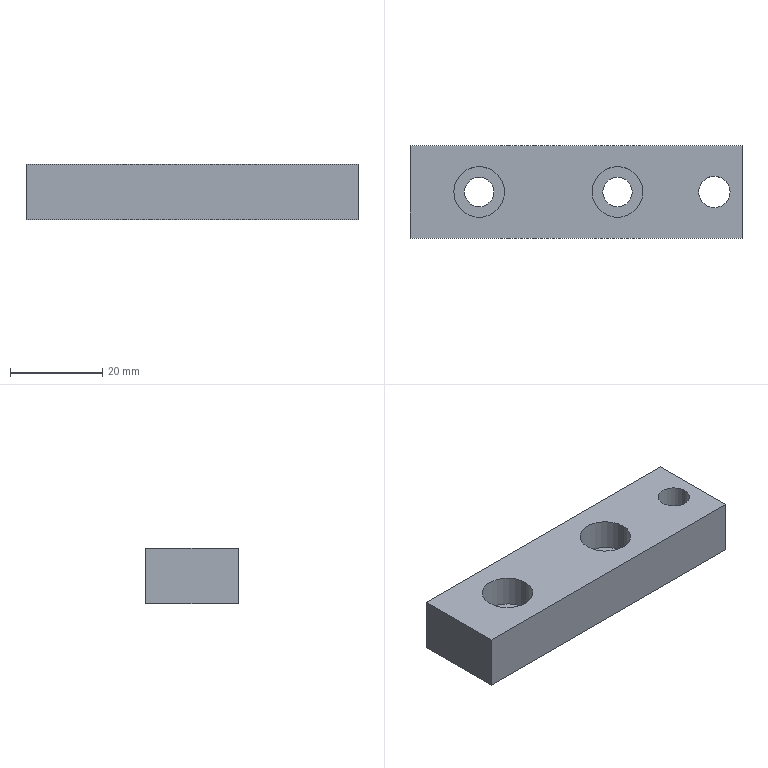Part | STEP file | Tensioning block | 1 solid | 18 faces | box 72 x 20 x 12 mm | volume 15217 mm3 | cylinder 10 | plane 8 | commonest cylinder face diameters 6.4 x4 11 x4 6.8 x2
STEP:
#1=CARTESIAN_POINT('',(0.,0.,0.));
#2=DIRECTION('',(0.,0.,1.));
#3=DIRECTION('',(1.,0.,0.));
#4=AXIS2_PLACEMENT_3D('',#1,#2,#3);
#5=CARTESIAN_POINT('',(33.4,0.,0.));
#6=VERTEX_POINT('',#5);
#7=CARTESIAN_POINT('',(33.4,0.,12.));
#8=VERTEX_POINT('',#7);
#9=CARTESIAN_POINT('',(33.4,0.,12.));
#10=DIRECTION('',(0.,0.,1.));
#11=VECTOR('',#10,1.);
#12=LINE('',#9,#11);
#13=CARTESIAN_POINT('',(30.,0.,12.));
#14=DIRECTION('',(0.,0.,1.));
#15=DIRECTION('',(1.,0.,0.));
#16=AXIS2_PLACEMENT_3D('',#13,#14,#15);
#17=CYLINDRICAL_SURFACE('',#16,3.4);
#18=CARTESIAN_POINT('',(6.283,0.));
#19=DIRECTION('',(0.,1.));
#20=VECTOR('',#19,1.);
#21=LINE('',#18,#20);
#22=(GEOMETRIC_REPRESENTATION_CONTEXT(2)PARAMETRIC_REPRESENTATION_CONTEXT()REPRESENTATION_CONTEXT('',''));
#23=DEFINITIONAL_REPRESENTATION('',(#21),#22);
#24=PCURVE('',#17,#23);
#25=CARTESIAN_POINT('',(30.,0.,12.));
#26=DIRECTION('',(0.,0.,1.));
#27=DIRECTION('',(1.,0.,0.));
#28=AXIS2_PLACEMENT_3D('',#25,#26,#27);
#29=CYLINDRICAL_SURFACE('',#28,3.4);
#30=CARTESIAN_POINT('',(0.,0.));
#31=DIRECTION('',(0.,1.));
#32=VECTOR('',#31,1.);
#33=LINE('',#30,#32);
#34=(GEOMETRIC_REPRESENTATION_CONTEXT(2)PARAMETRIC_REPRESENTATION_CONTEXT()REPRESENTATION_CONTEXT('',''));
#35=DEFINITIONAL_REPRESENTATION('',(#33),#34);
#36=PCURVE('',#29,#35);
#37=SURFACE_CURVE('',#12,(#24,#36),.PCURVE_S1.);
#38=EDGE_CURVE('',#6,#8,#37,.T.);
#39=ORIENTED_EDGE('',*,*,#38,.T.);
#40=CARTESIAN_POINT('',(26.6,0.,12.));
#41=VERTEX_POINT('',#40);
#42=CARTESIAN_POINT('',(30.,0.,12.));
#43=DIRECTION('',(0.,0.,1.));
#44=DIRECTION('',(1.,0.,0.));
#45=AXIS2_PLACEMENT_3D('',#42,#43,#44);
#46=CIRCLE('',#45,3.4);
#47=CARTESIAN_POINT('',(0.,0.));
#48=DIRECTION('',(1.,0.));
#49=VECTOR('',#48,1.);
#50=LINE('',#47,#49);
#51=(GEOMETRIC_REPRESENTATION_CONTEXT(2)PARAMETRIC_REPRESENTATION_CONTEXT()REPRESENTATION_CONTEXT('',''));
#52=DEFINITIONAL_REPRESENTATION('',(#50),#51);
#53=PCURVE('',#17,#52);
#54=CARTESIAN_POINT('',(0.,0.,12.));
#55=DIRECTION('',(0.,0.,1.));
#56=DIRECTION('',(1.,0.,0.));
#57=AXIS2_PLACEMENT_3D('',#54,#55,#56);
#58=PLANE('',#57);
#59=CARTESIAN_POINT('',(30.,0.));
#60=DIRECTION('',(1.,0.));
#61=AXIS2_PLACEMENT_2D('',#59,#60);
#62=CIRCLE('',#61,3.4);
#63=(GEOMETRIC_REPRESENTATION_CONTEXT(2)PARAMETRIC_REPRESENTATION_CONTEXT()REPRESENTATION_CONTEXT('',''));
#64=DEFINITIONAL_REPRESENTATION('',(#62),#63);
#65=PCURVE('',#58,#64);
#66=SURFACE_CURVE('',#46,(#53,#65),.PCURVE_S1.);
#67=EDGE_CURVE('',#41,#8,#66,.T.);
#68=ORIENTED_EDGE('',*,*,#67,.F.);
#69=CARTESIAN_POINT('',(26.6,0.,0.));
#70=VERTEX_POINT('',#69);
#71=CARTESIAN_POINT('',(26.6,0.,12.));
#72=DIRECTION('',(0.,0.,1.));
#73=VECTOR('',#72,1.);
#74=LINE('',#71,#73);
#75=CARTESIAN_POINT('',(3.142,0.));
#76=DIRECTION('',(0.,1.));
#77=VECTOR('',#76,1.);
#78=LINE('',#75,#77);
#79=(GEOMETRIC_REPRESENTATION_CONTEXT(2)PARAMETRIC_REPRESENTATION_CONTEXT()REPRESENTATION_CONTEXT('',''));
#80=DEFINITIONAL_REPRESENTATION('',(#78),#79);
#81=PCURVE('',#17,#80);
#82=CARTESIAN_POINT('',(3.142,0.));
#83=DIRECTION('',(0.,1.));
#84=VECTOR('',#83,1.);
#85=LINE('',#82,#84);
#86=(GEOMETRIC_REPRESENTATION_CONTEXT(2)PARAMETRIC_REPRESENTATION_CONTEXT()REPRESENTATION_CONTEXT('',''));
#87=DEFINITIONAL_REPRESENTATION('',(#85),#86);
#88=PCURVE('',#29,#87);
#89=SURFACE_CURVE('',#74,(#81,#88),.PCURVE_S1.);
#90=EDGE_CURVE('',#70,#41,#89,.T.);
#91=ORIENTED_EDGE('',*,*,#90,.F.);
#92=CARTESIAN_POINT('',(30.,0.,0.));
#93=DIRECTION('',(0.,0.,1.));
#94=DIRECTION('',(1.,0.,0.));
#95=AXIS2_PLACEMENT_3D('',#92,#93,#94);
#96=CIRCLE('',#95,3.4);
#97=CARTESIAN_POINT('',(0.,-12.));
#98=DIRECTION('',(1.,0.));
#99=VECTOR('',#98,1.);
#100=LINE('',#97,#99);
#101=(GEOMETRIC_REPRESENTATION_CONTEXT(2)PARAMETRIC_REPRESENTATION_CONTEXT()REPRESENTATION_CONTEXT('',''));
#102=DEFINITIONAL_REPRESENTATION('',(#100),#101);
#103=PCURVE('',#17,#102);
#104=CARTESIAN_POINT('',(0.,0.,0.));
#105=DIRECTION('',(0.,0.,1.));
#106=DIRECTION('',(1.,0.,0.));
#107=AXIS2_PLACEMENT_3D('',#104,#105,#106);
#108=PLANE('',#107);
#109=CARTESIAN_POINT('',(30.,0.));
#110=DIRECTION('',(1.,0.));
#111=AXIS2_PLACEMENT_2D('',#109,#110);
#112=CIRCLE('',#111,3.4);
#113=(GEOMETRIC_REPRESENTATION_CONTEXT(2)PARAMETRIC_REPRESENTATION_CONTEXT()REPRESENTATION_CONTEXT('',''));
#114=DEFINITIONAL_REPRESENTATION('',(#112),#113);
#115=PCURVE('',#108,#114);
#116=SURFACE_CURVE('',#96,(#103,#115),.PCURVE_S1.);
#117=EDGE_CURVE('',#70,#6,#116,.T.);
#118=ORIENTED_EDGE('',*,*,#117,.T.);
#119=EDGE_LOOP('',(#39,#68,#91,#118));
#120=FACE_BOUND('',#119,.F.);
#121=ADVANCED_FACE('',(#120),#17,.F.);
#122=CARTESIAN_POINT('',(-15.5,0.,5.2));
#123=VERTEX_POINT('',#122);
#124=CARTESIAN_POINT('',(-15.5,0.,12.));
#125=VERTEX_POINT('',#124);
#126=CARTESIAN_POINT('',(-15.5,0.,12.));
#127=DIRECTION('',(0.,0.,1.));
#128=VECTOR('',#127,1.);
#129=LINE('',#126,#128);
#130=CARTESIAN_POINT('',(-21.,0.,12.));
#131=DIRECTION('',(0.,0.,1.));
#132=DIRECTION('',(1.,0.,0.));
#133=AXIS2_PLACEMENT_3D('',#130,#131,#132);
#134=CYLINDRICAL_SURFACE('',#133,5.5);
#135=CARTESIAN_POINT('',(6.283,0.));
#136=DIRECTION('',(0.,1.));
#137=VECTOR('',#136,1.);
#138=LINE('',#135,#137);
#139=(GEOMETRIC_REPRESENTATION_CONTEXT(2)PARAMETRIC_REPRESENTATION_CONTEXT()REPRESENTATION_CONTEXT('',''));
#140=DEFINITIONAL_REPRESENTATION('',(#138),#139);
#141=PCURVE('',#134,#140);
#142=CARTESIAN_POINT('',(-21.,0.,12.));
#143=DIRECTION('',(0.,0.,1.));
#144=DIRECTION('',(1.,0.,0.));
#145=AXIS2_PLACEMENT_3D('',#142,#143,#144);
#146=CYLINDRICAL_SURFACE('',#145,5.5);
#147=CARTESIAN_POINT('',(0.,0.));
#148=DIRECTION('',(0.,1.));
#149=VECTOR('',#148,1.);
#150=LINE('',#147,#149);
#151=(GEOMETRIC_REPRESENTATION_CONTEXT(2)PARAMETRIC_REPRESENTATION_CONTEXT()REPRESENTATION_CONTEXT('',''));
#152=DEFINITIONAL_REPRESENTATION('',(#150),#151);
#153=PCURVE('',#146,#152);
#154=SURFACE_CURVE('',#129,(#141,#153),.PCURVE_S1.);
#155=EDGE_CURVE('',#123,#125,#154,.T.);
#156=ORIENTED_EDGE('',*,*,#155,.T.);
#157=CARTESIAN_POINT('',(-26.5,0.,12.));
#158=VERTEX_POINT('',#157);
#159=CARTESIAN_POINT('',(-21.,0.,12.));
#160=DIRECTION('',(0.,0.,1.));
#161=DIRECTION('',(1.,0.,0.));
#162=AXIS2_PLACEMENT_3D('',#159,#160,#161);
#163=CIRCLE('',#162,5.5);
#164=CARTESIAN_POINT('',(0.,0.));
#165=DIRECTION('',(1.,0.));
#166=VECTOR('',#165,1.);
#167=LINE('',#164,#166);
#168=(GEOMETRIC_REPRESENTATION_CONTEXT(2)PARAMETRIC_REPRESENTATION_CONTEXT()REPRESENTATION_CONTEXT('',''));
#169=DEFINITIONAL_REPRESENTATION('',(#167),#168);
#170=PCURVE('',#134,#169);
#171=CARTESIAN_POINT('',(-21.,0.));
#172=DIRECTION('',(1.,0.));
#173=AXIS2_PLACEMENT_2D('',#171,#172);
#174=CIRCLE('',#173,5.5);
#175=(GEOMETRIC_REPRESENTATION_CONTEXT(2)PARAMETRIC_REPRESENTATION_CONTEXT()REPRESENTATION_CONTEXT('',''));
#176=DEFINITIONAL_REPRESENTATION('',(#174),#175);
#177=PCURVE('',#58,#176);
#178=SURFACE_CURVE('',#163,(#170,#177),.PCURVE_S1.);
#179=EDGE_CURVE('',#158,#125,#178,.T.);
#180=ORIENTED_EDGE('',*,*,#179,.F.);
#181=CARTESIAN_POINT('',(-26.5,0.,5.2));
#182=VERTEX_POINT('',#181);
#183=CARTESIAN_POINT('',(-26.5,0.,12.));
#184=DIRECTION('',(0.,0.,1.));
#185=VECTOR('',#184,1.);
#186=LINE('',#183,#185);
#187=CARTESIAN_POINT('',(3.142,0.));
#188=DIRECTION('',(0.,1.));
#189=VECTOR('',#188,1.);
#190=LINE('',#187,#189);
#191=(GEOMETRIC_REPRESENTATION_CONTEXT(2)PARAMETRIC_REPRESENTATION_CONTEXT()REPRESENTATION_CONTEXT('',''));
#192=DEFINITIONAL_REPRESENTATION('',(#190),#191);
#193=PCURVE('',#134,#192);
#194=CARTESIAN_POINT('',(3.142,0.));
#195=DIRECTION('',(0.,1.));
#196=VECTOR('',#195,1.);
#197=LINE('',#194,#196);
#198=(GEOMETRIC_REPRESENTATION_CONTEXT(2)PARAMETRIC_REPRESENTATION_CONTEXT()REPRESENTATION_CONTEXT('',''));
#199=DEFINITIONAL_REPRESENTATION('',(#197),#198);
#200=PCURVE('',#146,#199);
#201=SURFACE_CURVE('',#186,(#193,#200),.PCURVE_S1.);
#202=EDGE_CURVE('',#182,#158,#201,.T.);
#203=ORIENTED_EDGE('',*,*,#202,.F.);
#204=CARTESIAN_POINT('',(-21.,0.,5.2));
#205=DIRECTION('',(0.,0.,1.));
#206=DIRECTION('',(1.,0.,0.));
#207=AXIS2_PLACEMENT_3D('',#204,#205,#206);
#208=CIRCLE('',#207,5.5);
#209=CARTESIAN_POINT('',(0.,-6.8));
#210=DIRECTION('',(1.,0.));
#211=VECTOR('',#210,1.);
#212=LINE('',#209,#211);
#213=(GEOMETRIC_REPRESENTATION_CONTEXT(2)PARAMETRIC_REPRESENTATION_CONTEXT()REPRESENTATION_CONTEXT('',''));
#214=DEFINITIONAL_REPRESENTATION('',(#212),#213);
#215=PCURVE('',#134,#214);
#216=CARTESIAN_POINT('',(-17.8,0.,5.2));
#217=DIRECTION('',(0.,0.,-1.));
#218=DIRECTION('',(-1.,0.,0.));
#219=AXIS2_PLACEMENT_3D('',#216,#217,#218);
#220=PLANE('',#219);
#221=CARTESIAN_POINT('',(-2.3,0.));
#222=CARTESIAN_POINT('',(-2.3,9.526));
#223=CARTESIAN_POINT('',(5.95,4.763));
#224=CARTESIAN_POINT('',(14.2,0.));
#225=CARTESIAN_POINT('',(5.95,-4.763));
#226=CARTESIAN_POINT('',(-2.3,-9.526));
#227=CARTESIAN_POINT('',(-2.3,0.));
#228=(BOUNDED_CURVE()B_SPLINE_CURVE(2,(#221,#222,#223,#224,#225,#226,#227),.UNSPECIFIED.,.T.,.F.)B_SPLINE_CURVE_WITH_KNOTS((1,2,2,2,2,1),(-2.094,0.,2.094,4.189,6.283,8.378),.UNSPECIFIED.)CURVE()GEOMETRIC_REPRESENTATION_ITEM()RATIONAL_B_SPLINE_CURVE((1.,0.5,1.,0.5,1.,0.5,1.))REPRESENTATION_ITEM(''));
#229=(GEOMETRIC_REPRESENTATION_CONTEXT(2)PARAMETRIC_REPRESENTATION_CONTEXT()REPRESENTATION_CONTEXT('',''));
#230=DEFINITIONAL_REPRESENTATION('',(#228),#229);
#231=PCURVE('',#220,#230);
#232=SURFACE_CURVE('',#208,(#215,#231),.PCURVE_S1.);
#233=EDGE_CURVE('',#182,#123,#232,.T.);
#234=ORIENTED_EDGE('',*,*,#233,.T.);
#235=EDGE_LOOP('',(#156,#180,#203,#234));
#236=FACE_BOUND('',#235,.F.);
#237=ADVANCED_FACE('',(#236),#134,.F.);
#238=CARTESIAN_POINT('',(-17.8,0.,0.));
#239=VERTEX_POINT('',#238);
#240=CARTESIAN_POINT('',(-17.8,0.,5.2));
#241=VERTEX_POINT('',#240);
#242=CARTESIAN_POINT('',(-17.8,0.,12.));
#243=DIRECTION('',(0.,0.,1.));
#244=VECTOR('',#243,1.);
#245=LINE('',#242,#244);
#246=CARTESIAN_POINT('',(-21.,0.,12.));
#247=DIRECTION('',(0.,0.,1.));
#248=DIRECTION('',(1.,0.,0.));
#249=AXIS2_PLACEMENT_3D('',#246,#247,#248);
#250=CYLINDRICAL_SURFACE('',#249,3.2);
#251=CARTESIAN_POINT('',(6.283,0.));
#252=DIRECTION('',(0.,1.));
#253=VECTOR('',#252,1.);
#254=LINE('',#251,#253);
#255=(GEOMETRIC_REPRESENTATION_CONTEXT(2)PARAMETRIC_REPRESENTATION_CONTEXT()REPRESENTATION_CONTEXT('',''));
#256=DEFINITIONAL_REPRESENTATION('',(#254),#255);
#257=PCURVE('',#250,#256);
#258=CARTESIAN_POINT('',(-21.,0.,12.));
#259=DIRECTION('',(0.,0.,1.));
#260=DIRECTION('',(1.,0.,0.));
#261=AXIS2_PLACEMENT_3D('',#258,#259,#260);
#262=CYLINDRICAL_SURFACE('',#261,3.2);
#263=CARTESIAN_POINT('',(0.,0.));
#264=DIRECTION('',(0.,1.));
#265=VECTOR('',#264,1.);
#266=LINE('',#263,#265);
#267=(GEOMETRIC_REPRESENTATION_CONTEXT(2)PARAMETRIC_REPRESENTATION_CONTEXT()REPRESENTATION_CONTEXT('',''));
#268=DEFINITIONAL_REPRESENTATION('',(#266),#267);
#269=PCURVE('',#262,#268);
#270=SURFACE_CURVE('',#245,(#257,#269),.PCURVE_S1.);
#271=EDGE_CURVE('',#239,#241,#270,.T.);
#272=ORIENTED_EDGE('',*,*,#271,.T.);
#273=CARTESIAN_POINT('',(-24.2,0.,5.2));
#274=VERTEX_POINT('',#273);
#275=CARTESIAN_POINT('',(-21.,0.,5.2));
#276=DIRECTION('',(0.,0.,1.));
#277=DIRECTION('',(1.,0.,0.));
#278=AXIS2_PLACEMENT_3D('',#275,#276,#277);
#279=CIRCLE('',#278,3.2);
#280=CARTESIAN_POINT('',(0.,-6.8));
#281=DIRECTION('',(1.,0.));
#282=VECTOR('',#281,1.);
#283=LINE('',#280,#282);
#284=(GEOMETRIC_REPRESENTATION_CONTEXT(2)PARAMETRIC_REPRESENTATION_CONTEXT()REPRESENTATION_CONTEXT('',''));
#285=DEFINITIONAL_REPRESENTATION('',(#283),#284);
#286=PCURVE('',#250,#285);
#287=CARTESIAN_POINT('',(0.,0.));
#288=CARTESIAN_POINT('',(0.,5.543));
#289=CARTESIAN_POINT('',(4.8,2.771));
#290=CARTESIAN_POINT('',(9.6,0.));
#291=CARTESIAN_POINT('',(4.8,-2.771));
#292=CARTESIAN_POINT('',(0.,-5.543));
#293=CARTESIAN_POINT('',(0.,0.));
#294=(BOUNDED_CURVE()B_SPLINE_CURVE(2,(#287,#288,#289,#290,#291,#292,#293),.UNSPECIFIED.,.T.,.F.)B_SPLINE_CURVE_WITH_KNOTS((1,2,2,2,2,1),(-2.094,0.,2.094,4.189,6.283,8.378),.UNSPECIFIED.)CURVE()GEOMETRIC_REPRESENTATION_ITEM()RATIONAL_B_SPLINE_CURVE((1.,0.5,1.,0.5,1.,0.5,1.))REPRESENTATION_ITEM(''));
#295=(GEOMETRIC_REPRESENTATION_CONTEXT(2)PARAMETRIC_REPRESENTATION_CONTEXT()REPRESENTATION_CONTEXT('',''));
#296=DEFINITIONAL_REPRESENTATION('',(#294),#295);
#297=PCURVE('',#220,#296);
#298=SURFACE_CURVE('',#279,(#286,#297),.PCURVE_S1.);
#299=EDGE_CURVE('',#274,#241,#298,.T.);
#300=ORIENTED_EDGE('',*,*,#299,.F.);
#301=CARTESIAN_POINT('',(-24.2,0.,0.));
#302=VERTEX_POINT('',#301);
#303=CARTESIAN_POINT('',(-24.2,0.,12.));
#304=DIRECTION('',(0.,0.,1.));
#305=VECTOR('',#304,1.);
#306=LINE('',#303,#305);
#307=CARTESIAN_POINT('',(3.142,0.));
#308=DIRECTION('',(0.,1.));
#309=VECTOR('',#308,1.);
#310=LINE('',#307,#309);
#311=(GEOMETRIC_REPRESENTATION_CONTEXT(2)PARAMETRIC_REPRESENTATION_CONTEXT()REPRESENTATION_CONTEXT('',''));
#312=DEFINITIONAL_REPRESENTATION('',(#310),#311);
#313=PCURVE('',#250,#312);
#314=CARTESIAN_POINT('',(3.142,0.));
#315=DIRECTION('',(0.,1.));
#316=VECTOR('',#315,1.);
#317=LINE('',#314,#316);
#318=(GEOMETRIC_REPRESENTATION_CONTEXT(2)PARAMETRIC_REPRESENTATION_CONTEXT()REPRESENTATION_CONTEXT('',''));
#319=DEFINITIONAL_REPRESENTATION('',(#317),#318);
#320=PCURVE('',#262,#319);
#321=SURFACE_CURVE('',#306,(#313,#320),.PCURVE_S1.);
#322=EDGE_CURVE('',#302,#274,#321,.T.);
#323=ORIENTED_EDGE('',*,*,#322,.F.);
#324=CARTESIAN_POINT('',(-21.,0.,0.));
#325=DIRECTION('',(0.,0.,1.));
#326=DIRECTION('',(1.,0.,0.));
#327=AXIS2_PLACEMENT_3D('',#324,#325,#326);
#328=CIRCLE('',#327,3.2);
#329=CARTESIAN_POINT('',(0.,-12.));
#330=DIRECTION('',(1.,0.));
#331=VECTOR('',#330,1.);
#332=LINE('',#329,#331);
#333=(GEOMETRIC_REPRESENTATION_CONTEXT(2)PARAMETRIC_REPRESENTATION_CONTEXT()REPRESENTATION_CONTEXT('',''));
#334=DEFINITIONAL_REPRESENTATION('',(#332),#333);
#335=PCURVE('',#250,#334);
#336=CARTESIAN_POINT('',(-21.,0.));
#337=DIRECTION('',(1.,0.));
#338=AXIS2_PLACEMENT_2D('',#336,#337);
#339=CIRCLE('',#338,3.2);
#340=(GEOMETRIC_REPRESENTATION_CONTEXT(2)PARAMETRIC_REPRESENTATION_CONTEXT()REPRESENTATION_CONTEXT('',''));
#341=DEFINITIONAL_REPRESENTATION('',(#339),#340);
#342=PCURVE('',#108,#341);
#343=SURFACE_CURVE('',#328,(#335,#342),.PCURVE_S1.);
#344=EDGE_CURVE('',#302,#239,#343,.T.);
#345=ORIENTED_EDGE('',*,*,#344,.T.);
#346=EDGE_LOOP('',(#272,#300,#323,#345));
#347=FACE_BOUND('',#346,.F.);
#348=ADVANCED_FACE('',(#347),#250,.F.);
#349=CARTESIAN_POINT('',(14.5,0.,5.2));
#350=VERTEX_POINT('',#349);
#351=CARTESIAN_POINT('',(14.5,0.,12.));
#352=VERTEX_POINT('',#351);
#353=CARTESIAN_POINT('',(14.5,0.,12.));
#354=DIRECTION('',(0.,0.,1.));
#355=VECTOR('',#354,1.);
#356=LINE('',#353,#355);
#357=CARTESIAN_POINT('',(9.,0.,12.));
#358=DIRECTION('',(0.,0.,1.));
#359=DIRECTION('',(1.,0.,0.));
#360=AXIS2_PLACEMENT_3D('',#357,#358,#359);
#361=CYLINDRICAL_SURFACE('',#360,5.5);
#362=CARTESIAN_POINT('',(6.283,0.));
#363=DIRECTION('',(0.,1.));
#364=VECTOR('',#363,1.);
#365=LINE('',#362,#364);
#366=(GEOMETRIC_REPRESENTATION_CONTEXT(2)PARAMETRIC_REPRESENTATION_CONTEXT()REPRESENTATION_CONTEXT('',''));
#367=DEFINITIONAL_REPRESENTATION('',(#365),#366);
#368=PCURVE('',#361,#367);
#369=CARTESIAN_POINT('',(9.,0.,12.));
#370=DIRECTION('',(0.,0.,1.));
#371=DIRECTION('',(1.,0.,0.));
#372=AXIS2_PLACEMENT_3D('',#369,#370,#371);
#373=CYLINDRICAL_SURFACE('',#372,5.5);
#374=CARTESIAN_POINT('',(0.,0.));
#375=DIRECTION('',(0.,1.));
#376=VECTOR('',#375,1.);
#377=LINE('',#374,#376);
#378=(GEOMETRIC_REPRESENTATION_CONTEXT(2)PARAMETRIC_REPRESENTATION_CONTEXT()REPRESENTATION_CONTEXT('',''));
#379=DEFINITIONAL_REPRESENTATION('',(#377),#378);
#380=PCURVE('',#373,#379);
#381=SURFACE_CURVE('',#356,(#368,#380),.PCURVE_S1.);
#382=EDGE_CURVE('',#350,#352,#381,.T.);
#383=ORIENTED_EDGE('',*,*,#382,.T.);
#384=CARTESIAN_POINT('',(3.5,0.,12.));
#385=VERTEX_POINT('',#384);
#386=CARTESIAN_POINT('',(9.,0.,12.));
#387=DIRECTION('',(0.,0.,1.));
#388=DIRECTION('',(1.,0.,0.));
#389=AXIS2_PLACEMENT_3D('',#386,#387,#388);
#390=CIRCLE('',#389,5.5);
#391=CARTESIAN_POINT('',(0.,0.));
#392=DIRECTION('',(1.,0.));
#393=VECTOR('',#392,1.);
#394=LINE('',#391,#393);
#395=(GEOMETRIC_REPRESENTATION_CONTEXT(2)PARAMETRIC_REPRESENTATION_CONTEXT()REPRESENTATION_CONTEXT('',''));
#396=DEFINITIONAL_REPRESENTATION('',(#394),#395);
#397=PCURVE('',#361,#396);
#398=CARTESIAN_POINT('',(9.,0.));
#399=DIRECTION('',(1.,0.));
#400=AXIS2_PLACEMENT_2D('',#398,#399);
#401=CIRCLE('',#400,5.5);
#402=(GEOMETRIC_REPRESENTATION_CONTEXT(2)PARAMETRIC_REPRESENTATION_CONTEXT()REPRESENTATION_CONTEXT('',''));
#403=DEFINITIONAL_REPRESENTATION('',(#401),#402);
#404=PCURVE('',#58,#403);
#405=SURFACE_CURVE('',#390,(#397,#404),.PCURVE_S1.);
#406=EDGE_CURVE('',#385,#352,#405,.T.);
#407=ORIENTED_EDGE('',*,*,#406,.F.);
#408=CARTESIAN_POINT('',(3.5,0.,5.2));
#409=VERTEX_POINT('',#408);
#410=CARTESIAN_POINT('',(3.5,0.,12.));
#411=DIRECTION('',(0.,0.,1.));
#412=VECTOR('',#411,1.);
#413=LINE('',#410,#412);
#414=CARTESIAN_POINT('',(3.142,0.));
#415=DIRECTION('',(0.,1.));
#416=VECTOR('',#415,1.);
#417=LINE('',#414,#416);
#418=(GEOMETRIC_REPRESENTATION_CONTEXT(2)PARAMETRIC_REPRESENTATION_CONTEXT()REPRESENTATION_CONTEXT('',''));
#419=DEFINITIONAL_REPRESENTATION('',(#417),#418);
#420=PCURVE('',#361,#419);
#421=CARTESIAN_POINT('',(3.142,0.));
#422=DIRECTION('',(0.,1.));
#423=VECTOR('',#422,1.);
#424=LINE('',#421,#423);
#425=(GEOMETRIC_REPRESENTATION_CONTEXT(2)PARAMETRIC_REPRESENTATION_CONTEXT()REPRESENTATION_CONTEXT('',''));
#426=DEFINITIONAL_REPRESENTATION('',(#424),#425);
#427=PCURVE('',#373,#426);
#428=SURFACE_CURVE('',#413,(#420,#427),.PCURVE_S1.);
#429=EDGE_CURVE('',#409,#385,#428,.T.);
#430=ORIENTED_EDGE('',*,*,#429,.F.);
#431=CARTESIAN_POINT('',(9.,0.,5.2));
#432=DIRECTION('',(0.,0.,1.));
#433=DIRECTION('',(1.,0.,0.));
#434=AXIS2_PLACEMENT_3D('',#431,#432,#433);
#435=CIRCLE('',#434,5.5);
#436=CARTESIAN_POINT('',(0.,-6.8));
#437=DIRECTION('',(1.,0.));
#438=VECTOR('',#437,1.);
#439=LINE('',#436,#438);
#440=(GEOMETRIC_REPRESENTATION_CONTEXT(2)PARAMETRIC_REPRESENTATION_CONTEXT()REPRESENTATION_CONTEXT('',''));
#441=DEFINITIONAL_REPRESENTATION('',(#439),#440);
#442=PCURVE('',#361,#441);
#443=CARTESIAN_POINT('',(12.2,0.,5.2));
#444=DIRECTION('',(0.,0.,-1.));
#445=DIRECTION('',(-1.,0.,0.));
#446=AXIS2_PLACEMENT_3D('',#443,#444,#445);
#447=PLANE('',#446);
#448=CARTESIAN_POINT('',(-2.3,0.));
#449=CARTESIAN_POINT('',(-2.3,9.526));
#450=CARTESIAN_POINT('',(5.95,4.763));
#451=CARTESIAN_POINT('',(14.2,0.));
#452=CARTESIAN_POINT('',(5.95,-4.763));
#453=CARTESIAN_POINT('',(-2.3,-9.526));
#454=CARTESIAN_POINT('',(-2.3,0.));
#455=(BOUNDED_CURVE()B_SPLINE_CURVE(2,(#448,#449,#450,#451,#452,#453,#454),.UNSPECIFIED.,.T.,.F.)B_SPLINE_CURVE_WITH_KNOTS((1,2,2,2,2,1),(-2.094,0.,2.094,4.189,6.283,8.378),.UNSPECIFIED.)CURVE()GEOMETRIC_REPRESENTATION_ITEM()RATIONAL_B_SPLINE_CURVE((1.,0.5,1.,0.5,1.,0.5,1.))REPRESENTATION_ITEM(''));
#456=(GEOMETRIC_REPRESENTATION_CONTEXT(2)PARAMETRIC_REPRESENTATION_CONTEXT()REPRESENTATION_CONTEXT('',''));
#457=DEFINITIONAL_REPRESENTATION('',(#455),#456);
#458=PCURVE('',#447,#457);
#459=SURFACE_CURVE('',#435,(#442,#458),.PCURVE_S1.);
#460=EDGE_CURVE('',#409,#350,#459,.T.);
#461=ORIENTED_EDGE('',*,*,#460,.T.);
#462=EDGE_LOOP('',(#383,#407,#430,#461));
#463=FACE_BOUND('',#462,.F.);
#464=ADVANCED_FACE('',(#463),#361,.F.);
#465=CARTESIAN_POINT('',(12.2,0.,0.));
#466=VERTEX_POINT('',#465);
#467=CARTESIAN_POINT('',(12.2,0.,5.2));
#468=VERTEX_POINT('',#467);
#469=CARTESIAN_POINT('',(12.2,0.,12.));
#470=DIRECTION('',(0.,0.,1.));
#471=VECTOR('',#470,1.);
#472=LINE('',#469,#471);
#473=CARTESIAN_POINT('',(9.,0.,12.));
#474=DIRECTION('',(0.,0.,1.));
#475=DIRECTION('',(1.,0.,0.));
#476=AXIS2_PLACEMENT_3D('',#473,#474,#475);
#477=CYLINDRICAL_SURFACE('',#476,3.2);
#478=CARTESIAN_POINT('',(6.283,0.));
#479=DIRECTION('',(0.,1.));
#480=VECTOR('',#479,1.);
#481=LINE('',#478,#480);
#482=(GEOMETRIC_REPRESENTATION_CONTEXT(2)PARAMETRIC_REPRESENTATION_CONTEXT()REPRESENTATION_CONTEXT('',''));
#483=DEFINITIONAL_REPRESENTATION('',(#481),#482);
#484=PCURVE('',#477,#483);
#485=CARTESIAN_POINT('',(9.,0.,12.));
#486=DIRECTION('',(0.,0.,1.));
#487=DIRECTION('',(1.,0.,0.));
#488=AXIS2_PLACEMENT_3D('',#485,#486,#487);
#489=CYLINDRICAL_SURFACE('',#488,3.2);
#490=CARTESIAN_POINT('',(0.,0.));
#491=DIRECTION('',(0.,1.));
#492=VECTOR('',#491,1.);
#493=LINE('',#490,#492);
#494=(GEOMETRIC_REPRESENTATION_CONTEXT(2)PARAMETRIC_REPRESENTATION_CONTEXT()REPRESENTATION_CONTEXT('',''));
#495=DEFINITIONAL_REPRESENTATION('',(#493),#494);
#496=PCURVE('',#489,#495);
#497=SURFACE_CURVE('',#472,(#484,#496),.PCURVE_S1.);
#498=EDGE_CURVE('',#466,#468,#497,.T.);
#499=ORIENTED_EDGE('',*,*,#498,.T.);
#500=CARTESIAN_POINT('',(5.8,0.,5.2));
#501=VERTEX_POINT('',#500);
#502=CARTESIAN_POINT('',(9.,0.,5.2));
#503=DIRECTION('',(0.,0.,1.));
#504=DIRECTION('',(1.,0.,0.));
#505=AXIS2_PLACEMENT_3D('',#502,#503,#504);
#506=CIRCLE('',#505,3.2);
#507=CARTESIAN_POINT('',(0.,-6.8));
#508=DIRECTION('',(1.,0.));
#509=VECTOR('',#508,1.);
#510=LINE('',#507,#509);
#511=(GEOMETRIC_REPRESENTATION_CONTEXT(2)PARAMETRIC_REPRESENTATION_CONTEXT()REPRESENTATION_CONTEXT('',''));
#512=DEFINITIONAL_REPRESENTATION('',(#510),#511);
#513=PCURVE('',#477,#512);
#514=CARTESIAN_POINT('',(0.,0.));
#515=CARTESIAN_POINT('',(0.,5.543));
#516=CARTESIAN_POINT('',(4.8,2.771));
#517=CARTESIAN_POINT('',(9.6,0.));
#518=CARTESIAN_POINT('',(4.8,-2.771));
#519=CARTESIAN_POINT('',(0.,-5.543));
#520=CARTESIAN_POINT('',(0.,0.));
#521=(BOUNDED_CURVE()B_SPLINE_CURVE(2,(#514,#515,#516,#517,#518,#519,#520),.UNSPECIFIED.,.T.,.F.)B_SPLINE_CURVE_WITH_KNOTS((1,2,2,2,2,1),(-2.094,0.,2.094,4.189,6.283,8.378),.UNSPECIFIED.)CURVE()GEOMETRIC_REPRESENTATION_ITEM()RATIONAL_B_SPLINE_CURVE((1.,0.5,1.,0.5,1.,0.5,1.))REPRESENTATION_ITEM(''));
#522=(GEOMETRIC_REPRESENTATION_CONTEXT(2)PARAMETRIC_REPRESENTATION_CONTEXT()REPRESENTATION_CONTEXT('',''));
#523=DEFINITIONAL_REPRESENTATION('',(#521),#522);
#524=PCURVE('',#447,#523);
#525=SURFACE_CURVE('',#506,(#513,#524),.PCURVE_S1.);
#526=EDGE_CURVE('',#501,#468,#525,.T.);
#527=ORIENTED_EDGE('',*,*,#526,.F.);
#528=CARTESIAN_POINT('',(5.8,0.,0.));
#529=VERTEX_POINT('',#528);
#530=CARTESIAN_POINT('',(5.8,0.,12.));
#531=DIRECTION('',(0.,0.,1.));
#532=VECTOR('',#531,1.);
#533=LINE('',#530,#532);
#534=CARTESIAN_POINT('',(3.142,0.));
#535=DIRECTION('',(0.,1.));
#536=VECTOR('',#535,1.);
#537=LINE('',#534,#536);
#538=(GEOMETRIC_REPRESENTATION_CONTEXT(2)PARAMETRIC_REPRESENTATION_CONTEXT()REPRESENTATION_CONTEXT('',''));
#539=DEFINITIONAL_REPRESENTATION('',(#537),#538);
#540=PCURVE('',#477,#539);
#541=CARTESIAN_POINT('',(3.142,0.));
#542=DIRECTION('',(0.,1.));
#543=VECTOR('',#542,1.);
#544=LINE('',#541,#543);
#545=(GEOMETRIC_REPRESENTATION_CONTEXT(2)PARAMETRIC_REPRESENTATION_CONTEXT()REPRESENTATION_CONTEXT('',''));
#546=DEFINITIONAL_REPRESENTATION('',(#544),#545);
#547=PCURVE('',#489,#546);
#548=SURFACE_CURVE('',#533,(#540,#547),.PCURVE_S1.);
#549=EDGE_CURVE('',#529,#501,#548,.T.);
#550=ORIENTED_EDGE('',*,*,#549,.F.);
#551=CARTESIAN_POINT('',(9.,0.,0.));
#552=DIRECTION('',(0.,0.,1.));
#553=DIRECTION('',(1.,0.,0.));
#554=AXIS2_PLACEMENT_3D('',#551,#552,#553);
#555=CIRCLE('',#554,3.2);
#556=CARTESIAN_POINT('',(0.,-12.));
#557=DIRECTION('',(1.,0.));
#558=VECTOR('',#557,1.);
#559=LINE('',#556,#558);
#560=(GEOMETRIC_REPRESENTATION_CONTEXT(2)PARAMETRIC_REPRESENTATION_CONTEXT()REPRESENTATION_CONTEXT('',''));
#561=DEFINITIONAL_REPRESENTATION('',(#559),#560);
#562=PCURVE('',#477,#561);
#563=CARTESIAN_POINT('',(9.,0.));
#564=DIRECTION('',(1.,0.));
#565=AXIS2_PLACEMENT_2D('',#563,#564);
#566=CIRCLE('',#565,3.2);
#567=(GEOMETRIC_REPRESENTATION_CONTEXT(2)PARAMETRIC_REPRESENTATION_CONTEXT()REPRESENTATION_CONTEXT('',''));
#568=DEFINITIONAL_REPRESENTATION('',(#566),#567);
#569=PCURVE('',#108,#568);
#570=SURFACE_CURVE('',#555,(#562,#569),.PCURVE_S1.);
#571=EDGE_CURVE('',#529,#466,#570,.T.);
#572=ORIENTED_EDGE('',*,*,#571,.T.);
#573=EDGE_LOOP('',(#499,#527,#550,#572));
#574=FACE_BOUND('',#573,.F.);
#575=ADVANCED_FACE('',(#574),#477,.F.);
#576=CARTESIAN_POINT('',(36.,-10.,0.));
#577=VERTEX_POINT('',#576);
#578=CARTESIAN_POINT('',(36.,10.,0.));
#579=VERTEX_POINT('',#578);
#580=CARTESIAN_POINT('',(36.,10.,0.));
#581=DIRECTION('',(0.,1.,0.));
#582=VECTOR('',#581,1.);
#583=LINE('',#580,#582);
#584=CARTESIAN_POINT('',(36.,10.,12.));
#585=DIRECTION('',(-1.,0.,0.));
#586=DIRECTION('',(0.,0.,1.));
#587=AXIS2_PLACEMENT_3D('',#584,#585,#586);
#588=PLANE('',#587);
#589=CARTESIAN_POINT('',(-12.,0.));
#590=DIRECTION('',(0.,1.));
#591=VECTOR('',#590,1.);
#592=LINE('',#589,#591);
#593=(GEOMETRIC_REPRESENTATION_CONTEXT(2)PARAMETRIC_REPRESENTATION_CONTEXT()REPRESENTATION_CONTEXT('',''));
#594=DEFINITIONAL_REPRESENTATION('',(#592),#593);
#595=PCURVE('',#588,#594);
#596=CARTESIAN_POINT('',(36.,10.));
#597=DIRECTION('',(0.,1.));
#598=VECTOR('',#597,1.);
#599=LINE('',#596,#598);
#600=(GEOMETRIC_REPRESENTATION_CONTEXT(2)PARAMETRIC_REPRESENTATION_CONTEXT()REPRESENTATION_CONTEXT('',''));
#601=DEFINITIONAL_REPRESENTATION('',(#599),#600);
#602=PCURVE('',#108,#601);
#603=SURFACE_CURVE('',#583,(#595,#602),.PCURVE_S1.);
#604=EDGE_CURVE('',#577,#579,#603,.T.);
#605=ORIENTED_EDGE('',*,*,#604,.T.);
#606=CARTESIAN_POINT('',(36.,10.,12.));
#607=VERTEX_POINT('',#606);
#608=CARTESIAN_POINT('',(36.,10.,12.));
#609=DIRECTION('',(0.,0.,-1.));
#610=VECTOR('',#609,1.);
#611=LINE('',#608,#610);
#612=CARTESIAN_POINT('',(0.,0.));
#613=DIRECTION('',(-1.,0.));
#614=VECTOR('',#613,1.);
#615=LINE('',#612,#614);
#616=(GEOMETRIC_REPRESENTATION_CONTEXT(2)PARAMETRIC_REPRESENTATION_CONTEXT()REPRESENTATION_CONTEXT('',''));
#617=DEFINITIONAL_REPRESENTATION('',(#615),#616);
#618=PCURVE('',#588,#617);
#619=CARTESIAN_POINT('',(-36.,10.,12.));
#620=DIRECTION('',(0.,-1.,0.));
#621=DIRECTION('',(0.,0.,-1.));
#622=AXIS2_PLACEMENT_3D('',#619,#620,#621);
#623=PLANE('',#622);
#624=CARTESIAN_POINT('',(0.,72.));
#625=DIRECTION('',(1.,0.));
#626=VECTOR('',#625,1.);
#627=LINE('',#624,#626);
#628=(GEOMETRIC_REPRESENTATION_CONTEXT(2)PARAMETRIC_REPRESENTATION_CONTEXT()REPRESENTATION_CONTEXT('',''));
#629=DEFINITIONAL_REPRESENTATION('',(#627),#628);
#630=PCURVE('',#623,#629);
#631=SURFACE_CURVE('',#611,(#618,#630),.PCURVE_S1.);
#632=EDGE_CURVE('',#607,#579,#631,.T.);
#633=ORIENTED_EDGE('',*,*,#632,.F.);
#634=CARTESIAN_POINT('',(36.,-10.,12.));
#635=VERTEX_POINT('',#634);
#636=CARTESIAN_POINT('',(36.,10.,12.));
#637=DIRECTION('',(0.,1.,0.));
#638=VECTOR('',#637,1.);
#639=LINE('',#636,#638);
#640=CARTESIAN_POINT('',(0.,0.));
#641=DIRECTION('',(0.,1.));
#642=VECTOR('',#641,1.);
#643=LINE('',#640,#642);
#644=(GEOMETRIC_REPRESENTATION_CONTEXT(2)PARAMETRIC_REPRESENTATION_CONTEXT()REPRESENTATION_CONTEXT('',''));
#645=DEFINITIONAL_REPRESENTATION('',(#643),#644);
#646=PCURVE('',#588,#645);
#647=CARTESIAN_POINT('',(36.,10.));
#648=DIRECTION('',(0.,1.));
#649=VECTOR('',#648,1.);
#650=LINE('',#647,#649);
#651=(GEOMETRIC_REPRESENTATION_CONTEXT(2)PARAMETRIC_REPRESENTATION_CONTEXT()REPRESENTATION_CONTEXT('',''));
#652=DEFINITIONAL_REPRESENTATION('',(#650),#651);
#653=PCURVE('',#58,#652);
#654=SURFACE_CURVE('',#639,(#646,#653),.PCURVE_S1.);
#655=EDGE_CURVE('',#635,#607,#654,.T.);
#656=ORIENTED_EDGE('',*,*,#655,.F.);
#657=CARTESIAN_POINT('',(36.,-10.,12.));
#658=DIRECTION('',(0.,0.,-1.));
#659=VECTOR('',#658,1.);
#660=LINE('',#657,#659);
#661=CARTESIAN_POINT('',(0.,-20.));
#662=DIRECTION('',(-1.,0.));
#663=VECTOR('',#662,1.);
#664=LINE('',#661,#663);
#665=(GEOMETRIC_REPRESENTATION_CONTEXT(2)PARAMETRIC_REPRESENTATION_CONTEXT()REPRESENTATION_CONTEXT('',''));
#666=DEFINITIONAL_REPRESENTATION('',(#664),#665);
#667=PCURVE('',#588,#666);
#668=CARTESIAN_POINT('',(-36.,-10.,12.));
#669=DIRECTION('',(0.,1.,0.));
#670=DIRECTION('',(0.,0.,1.));
#671=AXIS2_PLACEMENT_3D('',#668,#669,#670);
#672=PLANE('',#671);
#673=CARTESIAN_POINT('',(0.,72.));
#674=DIRECTION('',(-1.,0.));
#675=VECTOR('',#674,1.);
#676=LINE('',#673,#675);
#677=(GEOMETRIC_REPRESENTATION_CONTEXT(2)PARAMETRIC_REPRESENTATION_CONTEXT()REPRESENTATION_CONTEXT('',''));
#678=DEFINITIONAL_REPRESENTATION('',(#676),#677);
#679=PCURVE('',#672,#678);
#680=SURFACE_CURVE('',#660,(#667,#679),.PCURVE_S1.);
#681=EDGE_CURVE('',#635,#577,#680,.T.);
#682=ORIENTED_EDGE('',*,*,#681,.T.);
#683=EDGE_LOOP('',(#605,#633,#656,#682));
#684=FACE_BOUND('',#683,.T.);
#685=ADVANCED_FACE('',(#684),#588,.F.);
#686=CARTESIAN_POINT('',(-36.,10.,0.));
#687=VERTEX_POINT('',#686);
#688=CARTESIAN_POINT('',(-36.,10.,0.));
#689=DIRECTION('',(-1.,0.,0.));
#690=VECTOR('',#689,1.);
#691=LINE('',#688,#690);
#692=CARTESIAN_POINT('',(12.,0.));
#693=DIRECTION('',(0.,-1.));
#694=VECTOR('',#693,1.);
#695=LINE('',#692,#694);
#696=(GEOMETRIC_REPRESENTATION_CONTEXT(2)PARAMETRIC_REPRESENTATION_CONTEXT()REPRESENTATION_CONTEXT('',''));
#697=DEFINITIONAL_REPRESENTATION('',(#695),#696);
#698=PCURVE('',#623,#697);
#699=CARTESIAN_POINT('',(-36.,10.));
#700=DIRECTION('',(-1.,0.));
#701=VECTOR('',#700,1.);
#702=LINE('',#699,#701);
#703=(GEOMETRIC_REPRESENTATION_CONTEXT(2)PARAMETRIC_REPRESENTATION_CONTEXT()REPRESENTATION_CONTEXT('',''));
#704=DEFINITIONAL_REPRESENTATION('',(#702),#703);
#705=PCURVE('',#108,#704);
#706=SURFACE_CURVE('',#691,(#698,#705),.PCURVE_S1.);
#707=EDGE_CURVE('',#579,#687,#706,.T.);
#708=ORIENTED_EDGE('',*,*,#707,.T.);
#709=CARTESIAN_POINT('',(-36.,10.,12.));
#710=VERTEX_POINT('',#709);
#711=CARTESIAN_POINT('',(-36.,10.,12.));
#712=DIRECTION('',(0.,0.,-1.));
#713=VECTOR('',#712,1.);
#714=LINE('',#711,#713);
#715=CARTESIAN_POINT('',(0.,0.));
#716=DIRECTION('',(1.,0.));
#717=VECTOR('',#716,1.);
#718=LINE('',#715,#717);
#719=(GEOMETRIC_REPRESENTATION_CONTEXT(2)PARAMETRIC_REPRESENTATION_CONTEXT()REPRESENTATION_CONTEXT('',''));
#720=DEFINITIONAL_REPRESENTATION('',(#718),#719);
#721=PCURVE('',#623,#720);
#722=CARTESIAN_POINT('',(-36.,10.,12.));
#723=DIRECTION('',(1.,0.,0.));
#724=DIRECTION('',(0.,1.,0.));
#725=AXIS2_PLACEMENT_3D('',#722,#723,#724);
#726=PLANE('',#725);
#727=CARTESIAN_POINT('',(0.,0.));
#728=DIRECTION('',(0.,-1.));
#729=VECTOR('',#728,1.);
#730=LINE('',#727,#729);
#731=(GEOMETRIC_REPRESENTATION_CONTEXT(2)PARAMETRIC_REPRESENTATION_CONTEXT()REPRESENTATION_CONTEXT('',''));
#732=DEFINITIONAL_REPRESENTATION('',(#730),#731);
#733=PCURVE('',#726,#732);
#734=SURFACE_CURVE('',#714,(#721,#733),.PCURVE_S1.);
#735=EDGE_CURVE('',#710,#687,#734,.T.);
#736=ORIENTED_EDGE('',*,*,#735,.F.);
#737=CARTESIAN_POINT('',(-36.,10.,12.));
#738=DIRECTION('',(-1.,0.,0.));
#739=VECTOR('',#738,1.);
#740=LINE('',#737,#739);
#741=CARTESIAN_POINT('',(0.,0.));
#742=DIRECTION('',(0.,-1.));
#743=VECTOR('',#742,1.);
#744=LINE('',#741,#743);
#745=(GEOMETRIC_REPRESENTATION_CONTEXT(2)PARAMETRIC_REPRESENTATION_CONTEXT()REPRESENTATION_CONTEXT('',''));
#746=DEFINITIONAL_REPRESENTATION('',(#744),#745);
#747=PCURVE('',#623,#746);
#748=CARTESIAN_POINT('',(-36.,10.));
#749=DIRECTION('',(-1.,0.));
#750=VECTOR('',#749,1.);
#751=LINE('',#748,#750);
#752=(GEOMETRIC_REPRESENTATION_CONTEXT(2)PARAMETRIC_REPRESENTATION_CONTEXT()REPRESENTATION_CONTEXT('',''));
#753=DEFINITIONAL_REPRESENTATION('',(#751),#752);
#754=PCURVE('',#58,#753);
#755=SURFACE_CURVE('',#740,(#747,#754),.PCURVE_S1.);
#756=EDGE_CURVE('',#607,#710,#755,.T.);
#757=ORIENTED_EDGE('',*,*,#756,.F.);
#758=ORIENTED_EDGE('',*,*,#632,.T.);
#759=EDGE_LOOP('',(#708,#736,#757,#758));
#760=FACE_BOUND('',#759,.T.);
#761=ADVANCED_FACE('',(#760),#623,.F.);
#762=CARTESIAN_POINT('',(-36.,-10.,0.));
#763=VERTEX_POINT('',#762);
#764=CARTESIAN_POINT('',(-36.,10.,0.));
#765=DIRECTION('',(0.,-1.,0.));
#766=VECTOR('',#765,1.);
#767=LINE('',#764,#766);
#768=CARTESIAN_POINT('',(0.,-12.));
#769=DIRECTION('',(-1.,0.));
#770=VECTOR('',#769,1.);
#771=LINE('',#768,#770);
#772=(GEOMETRIC_REPRESENTATION_CONTEXT(2)PARAMETRIC_REPRESENTATION_CONTEXT()REPRESENTATION_CONTEXT('',''));
#773=DEFINITIONAL_REPRESENTATION('',(#771),#772);
#774=PCURVE('',#726,#773);
#775=CARTESIAN_POINT('',(-36.,10.));
#776=DIRECTION('',(0.,-1.));
#777=VECTOR('',#776,1.);
#778=LINE('',#775,#777);
#779=(GEOMETRIC_REPRESENTATION_CONTEXT(2)PARAMETRIC_REPRESENTATION_CONTEXT()REPRESENTATION_CONTEXT('',''));
#780=DEFINITIONAL_REPRESENTATION('',(#778),#779);
#781=PCURVE('',#108,#780);
#782=SURFACE_CURVE('',#767,(#774,#781),.PCURVE_S1.);
#783=EDGE_CURVE('',#687,#763,#782,.T.);
#784=ORIENTED_EDGE('',*,*,#783,.T.);
#785=CARTESIAN_POINT('',(-36.,-10.,12.));
#786=VERTEX_POINT('',#785);
#787=CARTESIAN_POINT('',(-36.,-10.,12.));
#788=DIRECTION('',(0.,0.,-1.));
#789=VECTOR('',#788,1.);
#790=LINE('',#787,#789);
#791=CARTESIAN_POINT('',(-20.,0.));
#792=DIRECTION('',(0.,-1.));
#793=VECTOR('',#792,1.);
#794=LINE('',#791,#793);
#795=(GEOMETRIC_REPRESENTATION_CONTEXT(2)PARAMETRIC_REPRESENTATION_CONTEXT()REPRESENTATION_CONTEXT('',''));
#796=DEFINITIONAL_REPRESENTATION('',(#794),#795);
#797=PCURVE('',#726,#796);
#798=CARTESIAN_POINT('',(0.,0.));
#799=DIRECTION('',(-1.,0.));
#800=VECTOR('',#799,1.);
#801=LINE('',#798,#800);
#802=(GEOMETRIC_REPRESENTATION_CONTEXT(2)PARAMETRIC_REPRESENTATION_CONTEXT()REPRESENTATION_CONTEXT('',''));
#803=DEFINITIONAL_REPRESENTATION('',(#801),#802);
#804=PCURVE('',#672,#803);
#805=SURFACE_CURVE('',#790,(#797,#804),.PCURVE_S1.);
#806=EDGE_CURVE('',#786,#763,#805,.T.);
#807=ORIENTED_EDGE('',*,*,#806,.F.);
#808=CARTESIAN_POINT('',(-36.,10.,12.));
#809=DIRECTION('',(0.,-1.,0.));
#810=VECTOR('',#809,1.);
#811=LINE('',#808,#810);
#812=CARTESIAN_POINT('',(0.,0.));
#813=DIRECTION('',(-1.,0.));
#814=VECTOR('',#813,1.);
#815=LINE('',#812,#814);
#816=(GEOMETRIC_REPRESENTATION_CONTEXT(2)PARAMETRIC_REPRESENTATION_CONTEXT()REPRESENTATION_CONTEXT('',''));
#817=DEFINITIONAL_REPRESENTATION('',(#815),#816);
#818=PCURVE('',#726,#817);
#819=CARTESIAN_POINT('',(-36.,10.));
#820=DIRECTION('',(0.,-1.));
#821=VECTOR('',#820,1.);
#822=LINE('',#819,#821);
#823=(GEOMETRIC_REPRESENTATION_CONTEXT(2)PARAMETRIC_REPRESENTATION_CONTEXT()REPRESENTATION_CONTEXT('',''));
#824=DEFINITIONAL_REPRESENTATION('',(#822),#823);
#825=PCURVE('',#58,#824);
#826=SURFACE_CURVE('',#811,(#818,#825),.PCURVE_S1.);
#827=EDGE_CURVE('',#710,#786,#826,.T.);
#828=ORIENTED_EDGE('',*,*,#827,.F.);
#829=ORIENTED_EDGE('',*,*,#735,.T.);
#830=EDGE_LOOP('',(#784,#807,#828,#829));
#831=FACE_BOUND('',#830,.T.);
#832=ADVANCED_FACE('',(#831),#726,.F.);
#833=CARTESIAN_POINT('',(-36.,-10.,0.));
#834=DIRECTION('',(1.,0.,0.));
#835=VECTOR('',#834,1.);
#836=LINE('',#833,#835);
#837=CARTESIAN_POINT('',(-12.,0.));
#838=DIRECTION('',(0.,1.));
#839=VECTOR('',#838,1.);
#840=LINE('',#837,#839);
#841=(GEOMETRIC_REPRESENTATION_CONTEXT(2)PARAMETRIC_REPRESENTATION_CONTEXT()REPRESENTATION_CONTEXT('',''));
#842=DEFINITIONAL_REPRESENTATION('',(#840),#841);
#843=PCURVE('',#672,#842);
#844=CARTESIAN_POINT('',(-36.,-10.));
#845=DIRECTION('',(1.,0.));
#846=VECTOR('',#845,1.);
#847=LINE('',#844,#846);
#848=(GEOMETRIC_REPRESENTATION_CONTEXT(2)PARAMETRIC_REPRESENTATION_CONTEXT()REPRESENTATION_CONTEXT('',''));
#849=DEFINITIONAL_REPRESENTATION('',(#847),#848);
#850=PCURVE('',#108,#849);
#851=SURFACE_CURVE('',#836,(#843,#850),.PCURVE_S1.);
#852=EDGE_CURVE('',#763,#577,#851,.T.);
#853=ORIENTED_EDGE('',*,*,#852,.T.);
#854=ORIENTED_EDGE('',*,*,#681,.F.);
#855=CARTESIAN_POINT('',(-36.,-10.,12.));
#856=DIRECTION('',(1.,0.,0.));
#857=VECTOR('',#856,1.);
#858=LINE('',#855,#857);
#859=CARTESIAN_POINT('',(0.,0.));
#860=DIRECTION('',(0.,1.));
#861=VECTOR('',#860,1.);
#862=LINE('',#859,#861);
#863=(GEOMETRIC_REPRESENTATION_CONTEXT(2)PARAMETRIC_REPRESENTATION_CONTEXT()REPRESENTATION_CONTEXT('',''));
#864=DEFINITIONAL_REPRESENTATION('',(#862),#863);
#865=PCURVE('',#672,#864);
#866=CARTESIAN_POINT('',(-36.,-10.));
#867=DIRECTION('',(1.,0.));
#868=VECTOR('',#867,1.);
#869=LINE('',#866,#868);
#870=(GEOMETRIC_REPRESENTATION_CONTEXT(2)PARAMETRIC_REPRESENTATION_CONTEXT()REPRESENTATION_CONTEXT('',''));
#871=DEFINITIONAL_REPRESENTATION('',(#869),#870);
#872=PCURVE('',#58,#871);
#873=SURFACE_CURVE('',#858,(#865,#872),.PCURVE_S1.);
#874=EDGE_CURVE('',#786,#635,#873,.T.);
#875=ORIENTED_EDGE('',*,*,#874,.F.);
#876=ORIENTED_EDGE('',*,*,#806,.T.);
#877=EDGE_LOOP('',(#853,#854,#875,#876));
#878=FACE_BOUND('',#877,.T.);
#879=ADVANCED_FACE('',(#878),#672,.F.);
#880=CARTESIAN_POINT('',(30.,0.,12.));
#881=DIRECTION('',(0.,0.,1.));
#882=DIRECTION('',(1.,0.,0.));
#883=AXIS2_PLACEMENT_3D('',#880,#881,#882);
#884=CIRCLE('',#883,3.4);
#885=CARTESIAN_POINT('',(30.,0.));
#886=DIRECTION('',(1.,0.));
#887=AXIS2_PLACEMENT_2D('',#885,#886);
#888=CIRCLE('',#887,3.4);
#889=(GEOMETRIC_REPRESENTATION_CONTEXT(2)PARAMETRIC_REPRESENTATION_CONTEXT()REPRESENTATION_CONTEXT('',''));
#890=DEFINITIONAL_REPRESENTATION('',(#888),#889);
#891=PCURVE('',#58,#890);
#892=CARTESIAN_POINT('',(0.,0.));
#893=DIRECTION('',(1.,0.));
#894=VECTOR('',#893,1.);
#895=LINE('',#892,#894);
#896=(GEOMETRIC_REPRESENTATION_CONTEXT(2)PARAMETRIC_REPRESENTATION_CONTEXT()REPRESENTATION_CONTEXT('',''));
#897=DEFINITIONAL_REPRESENTATION('',(#895),#896);
#898=PCURVE('',#29,#897);
#899=SURFACE_CURVE('',#884,(#891,#898),.PCURVE_S1.);
#900=EDGE_CURVE('',#8,#41,#899,.T.);
#901=ORIENTED_EDGE('',*,*,#900,.F.);
#902=ORIENTED_EDGE('',*,*,#67,.F.);
#903=EDGE_LOOP('',(#901,#902));
#904=FACE_BOUND('',#903,.T.);
#905=CARTESIAN_POINT('',(-21.,0.,12.));
#906=DIRECTION('',(0.,0.,1.));
#907=DIRECTION('',(1.,0.,0.));
#908=AXIS2_PLACEMENT_3D('',#905,#906,#907);
#909=CIRCLE('',#908,5.5);
#910=CARTESIAN_POINT('',(-21.,0.));
#911=DIRECTION('',(1.,0.));
#912=AXIS2_PLACEMENT_2D('',#910,#911);
#913=CIRCLE('',#912,5.5);
#914=(GEOMETRIC_REPRESENTATION_CONTEXT(2)PARAMETRIC_REPRESENTATION_CONTEXT()REPRESENTATION_CONTEXT('',''));
#915=DEFINITIONAL_REPRESENTATION('',(#913),#914);
#916=PCURVE('',#58,#915);
#917=CARTESIAN_POINT('',(0.,0.));
#918=DIRECTION('',(1.,0.));
#919=VECTOR('',#918,1.);
#920=LINE('',#917,#919);
#921=(GEOMETRIC_REPRESENTATION_CONTEXT(2)PARAMETRIC_REPRESENTATION_CONTEXT()REPRESENTATION_CONTEXT('',''));
#922=DEFINITIONAL_REPRESENTATION('',(#920),#921);
#923=PCURVE('',#146,#922);
#924=SURFACE_CURVE('',#909,(#916,#923),.PCURVE_S1.);
#925=EDGE_CURVE('',#125,#158,#924,.T.);
#926=ORIENTED_EDGE('',*,*,#925,.F.);
#927=ORIENTED_EDGE('',*,*,#179,.F.);
#928=EDGE_LOOP('',(#926,#927));
#929=FACE_BOUND('',#928,.T.);
#930=CARTESIAN_POINT('',(9.,0.,12.));
#931=DIRECTION('',(0.,0.,1.));
#932=DIRECTION('',(1.,0.,0.));
#933=AXIS2_PLACEMENT_3D('',#930,#931,#932);
#934=CIRCLE('',#933,5.5);
#935=CARTESIAN_POINT('',(9.,0.));
#936=DIRECTION('',(1.,0.));
#937=AXIS2_PLACEMENT_2D('',#935,#936);
#938=CIRCLE('',#937,5.5);
#939=(GEOMETRIC_REPRESENTATION_CONTEXT(2)PARAMETRIC_REPRESENTATION_CONTEXT()REPRESENTATION_CONTEXT('',''));
#940=DEFINITIONAL_REPRESENTATION('',(#938),#939);
#941=PCURVE('',#58,#940);
#942=CARTESIAN_POINT('',(0.,0.));
#943=DIRECTION('',(1.,0.));
#944=VECTOR('',#943,1.);
#945=LINE('',#942,#944);
#946=(GEOMETRIC_REPRESENTATION_CONTEXT(2)PARAMETRIC_REPRESENTATION_CONTEXT()REPRESENTATION_CONTEXT('',''));
#947=DEFINITIONAL_REPRESENTATION('',(#945),#946);
#948=PCURVE('',#373,#947);
#949=SURFACE_CURVE('',#934,(#941,#948),.PCURVE_S1.);
#950=EDGE_CURVE('',#352,#385,#949,.T.);
#951=ORIENTED_EDGE('',*,*,#950,.F.);
#952=ORIENTED_EDGE('',*,*,#406,.F.);
#953=EDGE_LOOP('',(#951,#952));
#954=FACE_BOUND('',#953,.T.);
#955=ORIENTED_EDGE('',*,*,#655,.T.);
#956=ORIENTED_EDGE('',*,*,#756,.T.);
#957=ORIENTED_EDGE('',*,*,#827,.T.);
#958=ORIENTED_EDGE('',*,*,#874,.T.);
#959=EDGE_LOOP('',(#955,#956,#957,#958));
#960=FACE_BOUND('',#959,.T.);
#961=ADVANCED_FACE('',(#904,#929,#954,#960),#58,.T.);
#962=CARTESIAN_POINT('',(30.,0.,0.));
#963=DIRECTION('',(0.,0.,1.));
#964=DIRECTION('',(1.,0.,0.));
#965=AXIS2_PLACEMENT_3D('',#962,#963,#964);
#966=CIRCLE('',#965,3.4);
#967=CARTESIAN_POINT('',(30.,0.));
#968=DIRECTION('',(1.,0.));
#969=AXIS2_PLACEMENT_2D('',#967,#968);
#970=CIRCLE('',#969,3.4);
#971=(GEOMETRIC_REPRESENTATION_CONTEXT(2)PARAMETRIC_REPRESENTATION_CONTEXT()REPRESENTATION_CONTEXT('',''));
#972=DEFINITIONAL_REPRESENTATION('',(#970),#971);
#973=PCURVE('',#108,#972);
#974=CARTESIAN_POINT('',(0.,-12.));
#975=DIRECTION('',(1.,0.));
#976=VECTOR('',#975,1.);
#977=LINE('',#974,#976);
#978=(GEOMETRIC_REPRESENTATION_CONTEXT(2)PARAMETRIC_REPRESENTATION_CONTEXT()REPRESENTATION_CONTEXT('',''));
#979=DEFINITIONAL_REPRESENTATION('',(#977),#978);
#980=PCURVE('',#29,#979);
#981=SURFACE_CURVE('',#966,(#973,#980),.PCURVE_S1.);
#982=EDGE_CURVE('',#6,#70,#981,.T.);
#983=ORIENTED_EDGE('',*,*,#982,.T.);
#984=ORIENTED_EDGE('',*,*,#117,.T.);
#985=EDGE_LOOP('',(#983,#984));
#986=FACE_BOUND('',#985,.T.);
#987=CARTESIAN_POINT('',(-21.,0.,0.));
#988=DIRECTION('',(0.,0.,1.));
#989=DIRECTION('',(1.,0.,0.));
#990=AXIS2_PLACEMENT_3D('',#987,#988,#989);
#991=CIRCLE('',#990,3.2);
#992=CARTESIAN_POINT('',(-21.,0.));
#993=DIRECTION('',(1.,0.));
#994=AXIS2_PLACEMENT_2D('',#992,#993);
#995=CIRCLE('',#994,3.2);
#996=(GEOMETRIC_REPRESENTATION_CONTEXT(2)PARAMETRIC_REPRESENTATION_CONTEXT()REPRESENTATION_CONTEXT('',''));
#997=DEFINITIONAL_REPRESENTATION('',(#995),#996);
#998=PCURVE('',#108,#997);
#999=CARTESIAN_POINT('',(0.,-12.));
#1000=DIRECTION('',(1.,0.));
#1001=VECTOR('',#1000,1.);
#1002=LINE('',#999,#1001);
#1003=(GEOMETRIC_REPRESENTATION_CONTEXT(2)PARAMETRIC_REPRESENTATION_CONTEXT()REPRESENTATION_CONTEXT('',''));
#1004=DEFINITIONAL_REPRESENTATION('',(#1002),#1003);
#1005=PCURVE('',#262,#1004);
#1006=SURFACE_CURVE('',#991,(#998,#1005),.PCURVE_S1.);
#1007=EDGE_CURVE('',#239,#302,#1006,.T.);
#1008=ORIENTED_EDGE('',*,*,#1007,.T.);
#1009=ORIENTED_EDGE('',*,*,#344,.T.);
#1010=EDGE_LOOP('',(#1008,#1009));
#1011=FACE_BOUND('',#1010,.T.);
#1012=CARTESIAN_POINT('',(9.,0.,0.));
#1013=DIRECTION('',(0.,0.,1.));
#1014=DIRECTION('',(1.,0.,0.));
#1015=AXIS2_PLACEMENT_3D('',#1012,#1013,#1014);
#1016=CIRCLE('',#1015,3.2);
#1017=CARTESIAN_POINT('',(9.,0.));
#1018=DIRECTION('',(1.,0.));
#1019=AXIS2_PLACEMENT_2D('',#1017,#1018);
#1020=CIRCLE('',#1019,3.2);
#1021=(GEOMETRIC_REPRESENTATION_CONTEXT(2)PARAMETRIC_REPRESENTATION_CONTEXT()REPRESENTATION_CONTEXT('',''));
#1022=DEFINITIONAL_REPRESENTATION('',(#1020),#1021);
#1023=PCURVE('',#108,#1022);
#1024=CARTESIAN_POINT('',(0.,-12.));
#1025=DIRECTION('',(1.,0.));
#1026=VECTOR('',#1025,1.);
#1027=LINE('',#1024,#1026);
#1028=(GEOMETRIC_REPRESENTATION_CONTEXT(2)PARAMETRIC_REPRESENTATION_CONTEXT()REPRESENTATION_CONTEXT('',''));
#1029=DEFINITIONAL_REPRESENTATION('',(#1027),#1028);
#1030=PCURVE('',#489,#1029);
#1031=SURFACE_CURVE('',#1016,(#1023,#1030),.PCURVE_S1.);
#1032=EDGE_CURVE('',#466,#529,#1031,.T.);
#1033=ORIENTED_EDGE('',*,*,#1032,.T.);
#1034=ORIENTED_EDGE('',*,*,#571,.T.);
#1035=EDGE_LOOP('',(#1033,#1034));
#1036=FACE_BOUND('',#1035,.T.);
#1037=ORIENTED_EDGE('',*,*,#604,.F.);
#1038=ORIENTED_EDGE('',*,*,#852,.F.);
#1039=ORIENTED_EDGE('',*,*,#783,.F.);
#1040=ORIENTED_EDGE('',*,*,#707,.F.);
#1041=EDGE_LOOP('',(#1037,#1038,#1039,#1040));
#1042=FACE_BOUND('',#1041,.T.);
#1043=ADVANCED_FACE('',(#986,#1011,#1036,#1042),#108,.F.);
#1044=CARTESIAN_POINT('',(9.,0.,5.2));
#1045=DIRECTION('',(0.,0.,1.));
#1046=DIRECTION('',(1.,0.,0.));
#1047=AXIS2_PLACEMENT_3D('',#1044,#1045,#1046);
#1048=CIRCLE('',#1047,3.2);
#1049=CARTESIAN_POINT('',(0.,-6.8));
#1050=DIRECTION('',(1.,0.));
#1051=VECTOR('',#1050,1.);
#1052=LINE('',#1049,#1051);
#1053=(GEOMETRIC_REPRESENTATION_CONTEXT(2)PARAMETRIC_REPRESENTATION_CONTEXT()REPRESENTATION_CONTEXT('',''));
#1054=DEFINITIONAL_REPRESENTATION('',(#1052),#1053);
#1055=PCURVE('',#489,#1054);
#1056=CARTESIAN_POINT('',(0.,0.));
#1057=CARTESIAN_POINT('',(0.,5.543));
#1058=CARTESIAN_POINT('',(4.8,2.771));
#1059=CARTESIAN_POINT('',(9.6,0.));
#1060=CARTESIAN_POINT('',(4.8,-2.771));
#1061=CARTESIAN_POINT('',(0.,-5.543));
#1062=CARTESIAN_POINT('',(0.,0.));
#1063=(BOUNDED_CURVE()B_SPLINE_CURVE(2,(#1056,#1057,#1058,#1059,#1060,#1061,#1062),.UNSPECIFIED.,.T.,.F.)B_SPLINE_CURVE_WITH_KNOTS((1,2,2,2,2,1),(-2.094,0.,2.094,4.189,6.283,8.378),.UNSPECIFIED.)CURVE()GEOMETRIC_REPRESENTATION_ITEM()RATIONAL_B_SPLINE_CURVE((1.,0.5,1.,0.5,1.,0.5,1.))REPRESENTATION_ITEM(''));
#1064=(GEOMETRIC_REPRESENTATION_CONTEXT(2)PARAMETRIC_REPRESENTATION_CONTEXT()REPRESENTATION_CONTEXT('',''));
#1065=DEFINITIONAL_REPRESENTATION('',(#1063),#1064);
#1066=PCURVE('',#447,#1065);
#1067=SURFACE_CURVE('',#1048,(#1055,#1066),.PCURVE_S1.);
#1068=EDGE_CURVE('',#468,#501,#1067,.T.);
#1069=ORIENTED_EDGE('',*,*,#1068,.F.);
#1070=ORIENTED_EDGE('',*,*,#498,.F.);
#1071=ORIENTED_EDGE('',*,*,#1032,.T.);
#1072=ORIENTED_EDGE('',*,*,#549,.T.);
#1073=EDGE_LOOP('',(#1069,#1070,#1071,#1072));
#1074=FACE_BOUND('',#1073,.F.);
#1075=ADVANCED_FACE('',(#1074),#489,.F.);
#1076=ORIENTED_EDGE('',*,*,#1068,.F.);
#1077=ORIENTED_EDGE('',*,*,#526,.F.);
#1078=EDGE_LOOP('',(#1076,#1077));
#1079=FACE_BOUND('',#1078,.T.);
#1080=CARTESIAN_POINT('',(9.,0.,5.2));
#1081=DIRECTION('',(0.,0.,1.));
#1082=DIRECTION('',(1.,0.,0.));
#1083=AXIS2_PLACEMENT_3D('',#1080,#1081,#1082);
#1084=CIRCLE('',#1083,5.5);
#1085=CARTESIAN_POINT('',(-2.3,0.));
#1086=CARTESIAN_POINT('',(-2.3,9.526));
#1087=CARTESIAN_POINT('',(5.95,4.763));
#1088=CARTESIAN_POINT('',(14.2,0.));
#1089=CARTESIAN_POINT('',(5.95,-4.763));
#1090=CARTESIAN_POINT('',(-2.3,-9.526));
#1091=CARTESIAN_POINT('',(-2.3,0.));
#1092=(BOUNDED_CURVE()B_SPLINE_CURVE(2,(#1085,#1086,#1087,#1088,#1089,#1090,#1091),.UNSPECIFIED.,.T.,.F.)B_SPLINE_CURVE_WITH_KNOTS((1,2,2,2,2,1),(-2.094,0.,2.094,4.189,6.283,8.378),.UNSPECIFIED.)CURVE()GEOMETRIC_REPRESENTATION_ITEM()RATIONAL_B_SPLINE_CURVE((1.,0.5,1.,0.5,1.,0.5,1.))REPRESENTATION_ITEM(''));
#1093=(GEOMETRIC_REPRESENTATION_CONTEXT(2)PARAMETRIC_REPRESENTATION_CONTEXT()REPRESENTATION_CONTEXT('',''));
#1094=DEFINITIONAL_REPRESENTATION('',(#1092),#1093);
#1095=PCURVE('',#447,#1094);
#1096=CARTESIAN_POINT('',(0.,-6.8));
#1097=DIRECTION('',(1.,0.));
#1098=VECTOR('',#1097,1.);
#1099=LINE('',#1096,#1098);
#1100=(GEOMETRIC_REPRESENTATION_CONTEXT(2)PARAMETRIC_REPRESENTATION_CONTEXT()REPRESENTATION_CONTEXT('',''));
#1101=DEFINITIONAL_REPRESENTATION('',(#1099),#1100);
#1102=PCURVE('',#373,#1101);
#1103=SURFACE_CURVE('',#1084,(#1095,#1102),.PCURVE_S1.);
#1104=EDGE_CURVE('',#350,#409,#1103,.T.);
#1105=ORIENTED_EDGE('',*,*,#1104,.T.);
#1106=ORIENTED_EDGE('',*,*,#460,.T.);
#1107=EDGE_LOOP('',(#1105,#1106));
#1108=FACE_BOUND('',#1107,.T.);
#1109=ADVANCED_FACE('',(#1079,#1108),#447,.F.);
#1110=ORIENTED_EDGE('',*,*,#950,.F.);
#1111=ORIENTED_EDGE('',*,*,#382,.F.);
#1112=ORIENTED_EDGE('',*,*,#1104,.T.);
#1113=ORIENTED_EDGE('',*,*,#429,.T.);
#1114=EDGE_LOOP('',(#1110,#1111,#1112,#1113));
#1115=FACE_BOUND('',#1114,.F.);
#1116=ADVANCED_FACE('',(#1115),#373,.F.);
#1117=CARTESIAN_POINT('',(-21.,0.,5.2));
#1118=DIRECTION('',(0.,0.,1.));
#1119=DIRECTION('',(1.,0.,0.));
#1120=AXIS2_PLACEMENT_3D('',#1117,#1118,#1119);
#1121=CIRCLE('',#1120,3.2);
#1122=CARTESIAN_POINT('',(0.,-6.8));
#1123=DIRECTION('',(1.,0.));
#1124=VECTOR('',#1123,1.);
#1125=LINE('',#1122,#1124);
#1126=(GEOMETRIC_REPRESENTATION_CONTEXT(2)PARAMETRIC_REPRESENTATION_CONTEXT()REPRESENTATION_CONTEXT('',''));
#1127=DEFINITIONAL_REPRESENTATION('',(#1125),#1126);
#1128=PCURVE('',#262,#1127);
#1129=CARTESIAN_POINT('',(0.,0.));
#1130=CARTESIAN_POINT('',(0.,5.543));
#1131=CARTESIAN_POINT('',(4.8,2.771));
#1132=CARTESIAN_POINT('',(9.6,0.));
#1133=CARTESIAN_POINT('',(4.8,-2.771));
#1134=CARTESIAN_POINT('',(0.,-5.543));
#1135=CARTESIAN_POINT('',(0.,0.));
#1136=(BOUNDED_CURVE()B_SPLINE_CURVE(2,(#1129,#1130,#1131,#1132,#1133,#1134,#1135),.UNSPECIFIED.,.T.,.F.)B_SPLINE_CURVE_WITH_KNOTS((1,2,2,2,2,1),(-2.094,0.,2.094,4.189,6.283,8.378),.UNSPECIFIED.)CURVE()GEOMETRIC_REPRESENTATION_ITEM()RATIONAL_B_SPLINE_CURVE((1.,0.5,1.,0.5,1.,0.5,1.))REPRESENTATION_ITEM(''));
#1137=(GEOMETRIC_REPRESENTATION_CONTEXT(2)PARAMETRIC_REPRESENTATION_CONTEXT()REPRESENTATION_CONTEXT('',''));
#1138=DEFINITIONAL_REPRESENTATION('',(#1136),#1137);
#1139=PCURVE('',#220,#1138);
#1140=SURFACE_CURVE('',#1121,(#1128,#1139),.PCURVE_S1.);
#1141=EDGE_CURVE('',#241,#274,#1140,.T.);
#1142=ORIENTED_EDGE('',*,*,#1141,.F.);
#1143=ORIENTED_EDGE('',*,*,#271,.F.);
#1144=ORIENTED_EDGE('',*,*,#1007,.T.);
#1145=ORIENTED_EDGE('',*,*,#322,.T.);
#1146=EDGE_LOOP('',(#1142,#1143,#1144,#1145));
#1147=FACE_BOUND('',#1146,.F.);
#1148=ADVANCED_FACE('',(#1147),#262,.F.);
#1149=ORIENTED_EDGE('',*,*,#1141,.F.);
#1150=ORIENTED_EDGE('',*,*,#299,.F.);
#1151=EDGE_LOOP('',(#1149,#1150));
#1152=FACE_BOUND('',#1151,.T.);
#1153=CARTESIAN_POINT('',(-21.,0.,5.2));
#1154=DIRECTION('',(0.,0.,1.));
#1155=DIRECTION('',(1.,0.,0.));
#1156=AXIS2_PLACEMENT_3D('',#1153,#1154,#1155);
#1157=CIRCLE('',#1156,5.5);
#1158=CARTESIAN_POINT('',(-2.3,0.));
#1159=CARTESIAN_POINT('',(-2.3,9.526));
#1160=CARTESIAN_POINT('',(5.95,4.763));
#1161=CARTESIAN_POINT('',(14.2,0.));
#1162=CARTESIAN_POINT('',(5.95,-4.763));
#1163=CARTESIAN_POINT('',(-2.3,-9.526));
#1164=CARTESIAN_POINT('',(-2.3,0.));
#1165=(BOUNDED_CURVE()B_SPLINE_CURVE(2,(#1158,#1159,#1160,#1161,#1162,#1163,#1164),.UNSPECIFIED.,.T.,.F.)B_SPLINE_CURVE_WITH_KNOTS((1,2,2,2,2,1),(-2.094,0.,2.094,4.189,6.283,8.378),.UNSPECIFIED.)CURVE()GEOMETRIC_REPRESENTATION_ITEM()RATIONAL_B_SPLINE_CURVE((1.,0.5,1.,0.5,1.,0.5,1.))REPRESENTATION_ITEM(''));
#1166=(GEOMETRIC_REPRESENTATION_CONTEXT(2)PARAMETRIC_REPRESENTATION_CONTEXT()REPRESENTATION_CONTEXT('',''));
#1167=DEFINITIONAL_REPRESENTATION('',(#1165),#1166);
#1168=PCURVE('',#220,#1167);
#1169=CARTESIAN_POINT('',(0.,-6.8));
#1170=DIRECTION('',(1.,0.));
#1171=VECTOR('',#1170,1.);
#1172=LINE('',#1169,#1171);
#1173=(GEOMETRIC_REPRESENTATION_CONTEXT(2)PARAMETRIC_REPRESENTATION_CONTEXT()REPRESENTATION_CONTEXT('',''));
#1174=DEFINITIONAL_REPRESENTATION('',(#1172),#1173);
#1175=PCURVE('',#146,#1174);
#1176=SURFACE_CURVE('',#1157,(#1168,#1175),.PCURVE_S1.);
#1177=EDGE_CURVE('',#123,#182,#1176,.T.);
#1178=ORIENTED_EDGE('',*,*,#1177,.T.);
#1179=ORIENTED_EDGE('',*,*,#233,.T.);
#1180=EDGE_LOOP('',(#1178,#1179));
#1181=FACE_BOUND('',#1180,.T.);
#1182=ADVANCED_FACE('',(#1152,#1181),#220,.F.);
#1183=ORIENTED_EDGE('',*,*,#925,.F.);
#1184=ORIENTED_EDGE('',*,*,#155,.F.);
#1185=ORIENTED_EDGE('',*,*,#1177,.T.);
#1186=ORIENTED_EDGE('',*,*,#202,.T.);
#1187=EDGE_LOOP('',(#1183,#1184,#1185,#1186));
#1188=FACE_BOUND('',#1187,.F.);
#1189=ADVANCED_FACE('',(#1188),#146,.F.);
#1190=ORIENTED_EDGE('',*,*,#900,.F.);
#1191=ORIENTED_EDGE('',*,*,#38,.F.);
#1192=ORIENTED_EDGE('',*,*,#982,.T.);
#1193=ORIENTED_EDGE('',*,*,#90,.T.);
#1194=EDGE_LOOP('',(#1190,#1191,#1192,#1193));
#1195=FACE_BOUND('',#1194,.F.);
#1196=ADVANCED_FACE('',(#1195),#29,.F.);
#1197=CLOSED_SHELL('',(#121,#237,#348,#464,#575,#685,#761,#832,#879,#961,#1043,#1075,#1109,#1116,#1148,#1182,#1189,#1196));
#1198=MANIFOLD_SOLID_BREP('',#1197);
#1199=(LENGTH_UNIT()NAMED_UNIT(*)SI_UNIT(.MILLI.,.METRE.));
#1200=UNCERTAINTY_MEASURE_WITH_UNIT(LENGTH_MEASURE(0.0000001),#1199,'','');
#1201=(NAMED_UNIT(*)PLANE_ANGLE_UNIT()SI_UNIT($,.RADIAN.));
#1202=(NAMED_UNIT(*)SI_UNIT($,.STERADIAN.)SOLID_ANGLE_UNIT());
#1203=(GEOMETRIC_REPRESENTATION_CONTEXT(3)GLOBAL_UNCERTAINTY_ASSIGNED_CONTEXT((#1200))GLOBAL_UNIT_ASSIGNED_CONTEXT((#1199,#1201,#1202))REPRESENTATION_CONTEXT('',''));
#1204=ADVANCED_BREP_SHAPE_REPRESENTATION('',(#4,#1198),#1203);